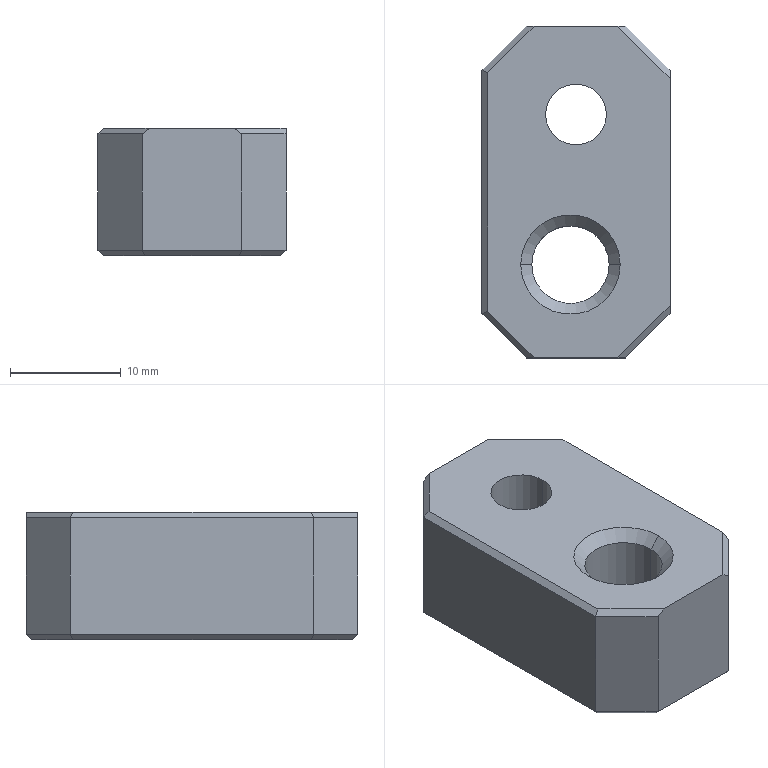Part | Creo | 1 solid | 34 faces | box 17 x 30 x 11.5 mm | volume 4458 mm3 | plane 24 | cylinder 6 | cone 4 | commonest cylinder face diameters 5.5 x2 7 x2 9.5 x2
STEP:
#1=CARTESIAN_POINT('',(-80.,-44.222,-93.5));
#2=VERTEX_POINT('',#1);
#3=CARTESIAN_POINT('',(-80.,-23.636,-93.5));
#4=VERTEX_POINT('',#3);
#5=CARTESIAN_POINT('',(-80.,-44.222,-93.5));
#6=DIRECTION('',(0.,1.,0.));
#7=VECTOR('',#6,20.586);
#8=LINE('',#5,#7);
#9=EDGE_CURVE('',#2,#4,#8,.T.);
#10=ORIENTED_EDGE('',*,*,#9,.F.);
#11=CARTESIAN_POINT('',(-84.707,-48.929,-93.5));
#12=VERTEX_POINT('',#11);
#13=CARTESIAN_POINT('',(-84.707,-48.929,-93.5));
#14=DIRECTION('',(0.7071,0.7071,0.));
#15=VECTOR('',#14,6.657);
#16=LINE('',#13,#15);
#17=EDGE_CURVE('',#12,#2,#16,.T.);
#18=ORIENTED_EDGE('',*,*,#17,.F.);
#19=CARTESIAN_POINT('',(-92.293,-48.929,-93.5));
#20=VERTEX_POINT('',#19);
#21=CARTESIAN_POINT('',(-92.293,-48.929,-93.5));
#22=DIRECTION('',(1.,0.,0.));
#23=VECTOR('',#22,7.586);
#24=LINE('',#21,#23);
#25=EDGE_CURVE('',#20,#12,#24,.T.);
#26=ORIENTED_EDGE('',*,*,#25,.F.);
#27=CARTESIAN_POINT('',(-96.5,-44.722,-93.5));
#28=VERTEX_POINT('',#27);
#29=CARTESIAN_POINT('',(-96.5,-44.722,-93.5));
#30=DIRECTION('',(0.7071,-0.7071,0.));
#31=VECTOR('',#30,5.95);
#32=LINE('',#29,#31);
#33=EDGE_CURVE('',#28,#20,#32,.T.);
#34=ORIENTED_EDGE('',*,*,#33,.F.);
#35=CARTESIAN_POINT('',(-96.5,-23.136,-93.5));
#36=VERTEX_POINT('',#35);
#37=CARTESIAN_POINT('',(-96.5,-44.722,-93.5));
#38=DIRECTION('',(0.,1.,0.));
#39=VECTOR('',#38,21.586);
#40=LINE('',#37,#39);
#41=EDGE_CURVE('',#28,#36,#40,.T.);
#42=ORIENTED_EDGE('',*,*,#41,.T.);
#43=CARTESIAN_POINT('',(-92.293,-18.929,-93.5));
#44=VERTEX_POINT('',#43);
#45=CARTESIAN_POINT('',(-92.293,-18.929,-93.5));
#46=DIRECTION('',(-0.7071,-0.7071,0.));
#47=VECTOR('',#46,5.95);
#48=LINE('',#45,#47);
#49=EDGE_CURVE('',#44,#36,#48,.T.);
#50=ORIENTED_EDGE('',*,*,#49,.F.);
#51=CARTESIAN_POINT('',(-84.707,-18.929,-93.5));
#52=VERTEX_POINT('',#51);
#53=CARTESIAN_POINT('',(-84.707,-18.929,-93.5));
#54=DIRECTION('',(-1.,0.,0.));
#55=VECTOR('',#54,7.586);
#56=LINE('',#53,#55);
#57=EDGE_CURVE('',#52,#44,#56,.T.);
#58=ORIENTED_EDGE('',*,*,#57,.F.);
#59=CARTESIAN_POINT('',(-80.,-23.636,-93.5));
#60=DIRECTION('',(-0.7071,0.7071,0.));
#61=VECTOR('',#60,6.657);
#62=LINE('',#59,#61);
#63=EDGE_CURVE('',#4,#52,#62,.T.);
#64=ORIENTED_EDGE('',*,*,#63,.F.);
#65=EDGE_LOOP('',(#10,#18,#26,#34,#42,#50,#58,#64));
#66=FACE_OUTER_BOUND('',#65,.F.);
#67=CARTESIAN_POINT('',(-91.25,-26.929,-93.5));
#68=VERTEX_POINT('',#67);
#69=CARTESIAN_POINT('',(-85.75,-26.929,-93.5));
#70=VERTEX_POINT('',#69);
#71=CARTESIAN_POINT('',(-88.5,-26.929,-93.5));
#72=DIRECTION('',(0.,0.,-1.));
#73=DIRECTION('',(-1.,0.,0.));
#74=AXIS2_PLACEMENT_3D('',#71,#72,#73);
#75=CIRCLE('',#74,2.75);
#76=EDGE_CURVE('',#68,#70,#75,.T.);
#77=ORIENTED_EDGE('',*,*,#76,.F.);
#78=CARTESIAN_POINT('',(-88.5,-26.929,-93.5));
#79=DIRECTION('',(0.,0.,-1.));
#80=DIRECTION('',(1.,0.,0.));
#81=AXIS2_PLACEMENT_3D('',#78,#79,#80);
#82=CIRCLE('',#81,2.75);
#83=EDGE_CURVE('',#70,#68,#82,.T.);
#84=ORIENTED_EDGE('',*,*,#83,.F.);
#85=EDGE_LOOP('',(#77,#84));
#86=FACE_BOUND('',#85,.F.);
#87=CARTESIAN_POINT('',(-84.5,-40.5,-93.5));
#88=VERTEX_POINT('',#87);
#89=CARTESIAN_POINT('',(-93.5,-40.5,-93.5));
#90=VERTEX_POINT('',#89);
#91=CARTESIAN_POINT('',(-89.,-40.5,-93.5));
#92=DIRECTION('',(0.,0.,-1.));
#93=DIRECTION('',(1.,0.,0.));
#94=AXIS2_PLACEMENT_3D('',#91,#92,#93);
#95=CIRCLE('',#94,4.5);
#96=EDGE_CURVE('',#88,#90,#95,.T.);
#97=ORIENTED_EDGE('',*,*,#96,.F.);
#98=CARTESIAN_POINT('',(-89.,-40.5,-93.5));
#99=DIRECTION('',(0.,0.,-1.));
#100=DIRECTION('',(-1.,0.,0.));
#101=AXIS2_PLACEMENT_3D('',#98,#99,#100);
#102=CIRCLE('',#101,4.5);
#103=EDGE_CURVE('',#90,#88,#102,.T.);
#104=ORIENTED_EDGE('',*,*,#103,.F.);
#105=EDGE_LOOP('',(#97,#104));
#106=FACE_BOUND('',#105,.F.);
#107=CARTESIAN_POINT('',(-88.428,-27.929,-93.5));
#108=DIRECTION('',(0.,0.,1.));
#109=DIRECTION('',(1.,0.,0.));
#110=AXIS2_PLACEMENT_3D('',#107,#108,#109);
#111=PLANE('',#110);
#112=ADVANCED_FACE('',(#66,#86,#106),#111,.T.);
#113=ORIENTED_EDGE('',*,*,#96,.T.);
#114=CARTESIAN_POINT('',(-92.5,-40.5,-94.5));
#115=VERTEX_POINT('',#114);
#116=CARTESIAN_POINT('',(-92.5,-40.5,-94.5));
#117=DIRECTION('',(-0.7071,0.,0.7071));
#118=VECTOR('',#117,1.414);
#119=LINE('',#116,#118);
#120=EDGE_CURVE('',#115,#90,#119,.T.);
#121=ORIENTED_EDGE('',*,*,#120,.F.);
#122=CARTESIAN_POINT('',(-85.5,-40.5,-94.5));
#123=VERTEX_POINT('',#122);
#124=CARTESIAN_POINT('',(-89.,-40.5,-94.5));
#125=DIRECTION('',(0.,0.,-1.));
#126=DIRECTION('',(1.,0.,0.));
#127=AXIS2_PLACEMENT_3D('',#124,#125,#126);
#128=CIRCLE('',#127,3.5);
#129=EDGE_CURVE('',#123,#115,#128,.T.);
#130=ORIENTED_EDGE('',*,*,#129,.F.);
#131=CARTESIAN_POINT('',(-85.5,-40.5,-94.5));
#132=DIRECTION('',(0.7071,0.,0.7071));
#133=VECTOR('',#132,1.414);
#134=LINE('',#131,#133);
#135=EDGE_CURVE('',#123,#88,#134,.T.);
#136=ORIENTED_EDGE('',*,*,#135,.T.);
#137=EDGE_LOOP('',(#113,#121,#130,#136));
#138=FACE_OUTER_BOUND('',#137,.F.);
#139=CARTESIAN_POINT('',(-89.,-40.5,-94.));
#140=DIRECTION('',(0.,0.,1.));
#141=DIRECTION('',(1.,0.,0.));
#142=AXIS2_PLACEMENT_3D('',#139,#140,#141);
#143=CONICAL_SURFACE('',#142,4.,45.);
#144=ADVANCED_FACE('',(#138),#143,.F.);
#145=ORIENTED_EDGE('',*,*,#103,.T.);
#146=ORIENTED_EDGE('',*,*,#135,.F.);
#147=CARTESIAN_POINT('',(-89.,-40.5,-94.5));
#148=DIRECTION('',(0.,0.,-1.));
#149=DIRECTION('',(-1.,0.,0.));
#150=AXIS2_PLACEMENT_3D('',#147,#148,#149);
#151=CIRCLE('',#150,3.5);
#152=EDGE_CURVE('',#115,#123,#151,.T.);
#153=ORIENTED_EDGE('',*,*,#152,.F.);
#154=ORIENTED_EDGE('',*,*,#120,.T.);
#155=EDGE_LOOP('',(#145,#146,#153,#154));
#156=FACE_OUTER_BOUND('',#155,.F.);
#157=CARTESIAN_POINT('',(-89.,-40.5,-94.));
#158=DIRECTION('',(0.,0.,1.));
#159=DIRECTION('',(1.,0.,0.));
#160=AXIS2_PLACEMENT_3D('',#157,#158,#159);
#161=CONICAL_SURFACE('',#160,4.,45.);
#162=ADVANCED_FACE('',(#156),#161,.F.);
#163=CARTESIAN_POINT('',(-85.5,-40.5,-104.));
#164=VERTEX_POINT('',#163);
#165=CARTESIAN_POINT('',(-92.5,-40.5,-104.));
#166=VERTEX_POINT('',#165);
#167=CARTESIAN_POINT('',(-89.,-40.5,-104.));
#168=DIRECTION('',(0.,0.,1.));
#169=DIRECTION('',(1.,0.,0.));
#170=AXIS2_PLACEMENT_3D('',#167,#168,#169);
#171=CIRCLE('',#170,3.5);
#172=EDGE_CURVE('',#164,#166,#171,.T.);
#173=ORIENTED_EDGE('',*,*,#172,.T.);
#174=CARTESIAN_POINT('',(-92.5,-40.5,-94.5));
#175=DIRECTION('',(0.,0.,-1.));
#176=VECTOR('',#175,9.5);
#177=LINE('',#174,#176);
#178=EDGE_CURVE('',#115,#166,#177,.T.);
#179=ORIENTED_EDGE('',*,*,#178,.F.);
#180=ORIENTED_EDGE('',*,*,#152,.T.);
#181=CARTESIAN_POINT('',(-85.5,-40.5,-94.5));
#182=DIRECTION('',(0.,0.,-1.));
#183=VECTOR('',#182,9.5);
#184=LINE('',#181,#183);
#185=EDGE_CURVE('',#123,#164,#184,.T.);
#186=ORIENTED_EDGE('',*,*,#185,.T.);
#187=EDGE_LOOP('',(#173,#179,#180,#186));
#188=FACE_OUTER_BOUND('',#187,.F.);
#189=CARTESIAN_POINT('',(-89.,-40.5,9.));
#190=DIRECTION('',(0.,0.,-1.));
#191=DIRECTION('',(1.,0.,0.));
#192=AXIS2_PLACEMENT_3D('',#189,#190,#191);
#193=CYLINDRICAL_SURFACE('',#192,3.5);
#194=ADVANCED_FACE('',(#188),#193,.F.);
#195=CARTESIAN_POINT('',(-84.5,-40.5,-105.));
#196=VERTEX_POINT('',#195);
#197=CARTESIAN_POINT('',(-93.5,-40.5,-105.));
#198=VERTEX_POINT('',#197);
#199=CARTESIAN_POINT('',(-89.,-40.5,-105.));
#200=DIRECTION('',(0.,0.,1.));
#201=DIRECTION('',(1.,0.,0.));
#202=AXIS2_PLACEMENT_3D('',#199,#200,#201);
#203=CIRCLE('',#202,4.5);
#204=EDGE_CURVE('',#196,#198,#203,.T.);
#205=ORIENTED_EDGE('',*,*,#204,.T.);
#206=CARTESIAN_POINT('',(-92.5,-40.5,-104.));
#207=DIRECTION('',(-0.7071,0.,-0.7071));
#208=VECTOR('',#207,1.414);
#209=LINE('',#206,#208);
#210=EDGE_CURVE('',#166,#198,#209,.T.);
#211=ORIENTED_EDGE('',*,*,#210,.F.);
#212=ORIENTED_EDGE('',*,*,#172,.F.);
#213=CARTESIAN_POINT('',(-85.5,-40.5,-104.));
#214=DIRECTION('',(0.7071,0.,-0.7071));
#215=VECTOR('',#214,1.414);
#216=LINE('',#213,#215);
#217=EDGE_CURVE('',#164,#196,#216,.T.);
#218=ORIENTED_EDGE('',*,*,#217,.T.);
#219=EDGE_LOOP('',(#205,#211,#212,#218));
#220=FACE_OUTER_BOUND('',#219,.F.);
#221=CARTESIAN_POINT('',(-89.,-40.5,-104.5));
#222=DIRECTION('',(0.,0.,-1.));
#223=DIRECTION('',(-1.,0.,0.));
#224=AXIS2_PLACEMENT_3D('',#221,#222,#223);
#225=CONICAL_SURFACE('',#224,4.,45.);
#226=ADVANCED_FACE('',(#220),#225,.F.);
#227=CARTESIAN_POINT('',(-80.5,-44.722,-105.));
#228=VERTEX_POINT('',#227);
#229=CARTESIAN_POINT('',(-80.5,-23.136,-105.));
#230=VERTEX_POINT('',#229);
#231=CARTESIAN_POINT('',(-80.5,-44.722,-105.));
#232=DIRECTION('',(0.,1.,0.));
#233=VECTOR('',#232,21.586);
#234=LINE('',#231,#233);
#235=EDGE_CURVE('',#228,#230,#234,.T.);
#236=ORIENTED_EDGE('',*,*,#235,.T.);
#237=CARTESIAN_POINT('',(-84.207,-19.429,-105.));
#238=VERTEX_POINT('',#237);
#239=CARTESIAN_POINT('',(-84.207,-19.429,-105.));
#240=DIRECTION('',(0.7071,-0.7071,0.));
#241=VECTOR('',#240,5.243);
#242=LINE('',#239,#241);
#243=EDGE_CURVE('',#238,#230,#242,.T.);
#244=ORIENTED_EDGE('',*,*,#243,.F.);
#245=CARTESIAN_POINT('',(-92.793,-19.429,-105.));
#246=VERTEX_POINT('',#245);
#247=CARTESIAN_POINT('',(-84.207,-19.429,-105.));
#248=DIRECTION('',(-1.,0.,0.));
#249=VECTOR('',#248,8.586);
#250=LINE('',#247,#249);
#251=EDGE_CURVE('',#238,#246,#250,.T.);
#252=ORIENTED_EDGE('',*,*,#251,.T.);
#253=CARTESIAN_POINT('',(-96.5,-23.136,-105.));
#254=VERTEX_POINT('',#253);
#255=CARTESIAN_POINT('',(-96.5,-23.136,-105.));
#256=DIRECTION('',(0.7071,0.7071,0.));
#257=VECTOR('',#256,5.243);
#258=LINE('',#255,#257);
#259=EDGE_CURVE('',#254,#246,#258,.T.);
#260=ORIENTED_EDGE('',*,*,#259,.F.);
#261=CARTESIAN_POINT('',(-96.5,-44.722,-105.));
#262=VERTEX_POINT('',#261);
#263=CARTESIAN_POINT('',(-96.5,-23.136,-105.));
#264=DIRECTION('',(0.,-1.,0.));
#265=VECTOR('',#264,21.586);
#266=LINE('',#263,#265);
#267=EDGE_CURVE('',#254,#262,#266,.T.);
#268=ORIENTED_EDGE('',*,*,#267,.T.);
#269=CARTESIAN_POINT('',(-92.793,-48.429,-105.));
#270=VERTEX_POINT('',#269);
#271=CARTESIAN_POINT('',(-92.793,-48.429,-105.));
#272=DIRECTION('',(-0.7071,0.7071,0.));
#273=VECTOR('',#272,5.243);
#274=LINE('',#271,#273);
#275=EDGE_CURVE('',#270,#262,#274,.T.);
#276=ORIENTED_EDGE('',*,*,#275,.F.);
#277=CARTESIAN_POINT('',(-84.207,-48.429,-105.));
#278=VERTEX_POINT('',#277);
#279=CARTESIAN_POINT('',(-92.793,-48.429,-105.));
#280=DIRECTION('',(1.,0.,0.));
#281=VECTOR('',#280,8.586);
#282=LINE('',#279,#281);
#283=EDGE_CURVE('',#270,#278,#282,.T.);
#284=ORIENTED_EDGE('',*,*,#283,.T.);
#285=CARTESIAN_POINT('',(-80.5,-44.722,-105.));
#286=DIRECTION('',(-0.7071,-0.7071,0.));
#287=VECTOR('',#286,5.243);
#288=LINE('',#285,#287);
#289=EDGE_CURVE('',#228,#278,#288,.T.);
#290=ORIENTED_EDGE('',*,*,#289,.F.);
#291=EDGE_LOOP('',(#236,#244,#252,#260,#268,#276,#284,#290));
#292=FACE_OUTER_BOUND('',#291,.F.);
#293=CARTESIAN_POINT('',(-83.75,-26.929,-105.));
#294=VERTEX_POINT('',#293);
#295=CARTESIAN_POINT('',(-93.25,-26.929,-105.));
#296=VERTEX_POINT('',#295);
#297=CARTESIAN_POINT('',(-88.5,-26.929,-105.));
#298=DIRECTION('',(0.,0.,1.));
#299=DIRECTION('',(1.,0.,0.));
#300=AXIS2_PLACEMENT_3D('',#297,#298,#299);
#301=CIRCLE('',#300,4.75);
#302=EDGE_CURVE('',#294,#296,#301,.T.);
#303=ORIENTED_EDGE('',*,*,#302,.F.);
#304=CARTESIAN_POINT('',(-88.5,-26.929,-105.));
#305=DIRECTION('',(0.,0.,1.));
#306=DIRECTION('',(-1.,0.,0.));
#307=AXIS2_PLACEMENT_3D('',#304,#305,#306);
#308=CIRCLE('',#307,4.75);
#309=EDGE_CURVE('',#296,#294,#308,.T.);
#310=ORIENTED_EDGE('',*,*,#309,.F.);
#311=EDGE_LOOP('',(#303,#310));
#312=FACE_BOUND('',#311,.F.);
#313=CARTESIAN_POINT('',(-89.,-40.5,-105.));
#314=DIRECTION('',(0.,0.,1.));
#315=DIRECTION('',(-1.,0.,0.));
#316=AXIS2_PLACEMENT_3D('',#313,#314,#315);
#317=CIRCLE('',#316,4.5);
#318=EDGE_CURVE('',#198,#196,#317,.T.);
#319=ORIENTED_EDGE('',*,*,#318,.F.);
#320=ORIENTED_EDGE('',*,*,#204,.F.);
#321=EDGE_LOOP('',(#319,#320));
#322=FACE_BOUND('',#321,.F.);
#323=CARTESIAN_POINT('',(-176.,-14.505,-105.));
#324=DIRECTION('',(0.,0.,-1.));
#325=DIRECTION('',(-1.,0.,0.));
#326=AXIS2_PLACEMENT_3D('',#323,#324,#325);
#327=PLANE('',#326);
#328=ADVANCED_FACE('',(#292,#312,#322),#327,.T.);
#329=ORIENTED_EDGE('',*,*,#318,.T.);
#330=ORIENTED_EDGE('',*,*,#217,.F.);
#331=CARTESIAN_POINT('',(-89.,-40.5,-104.));
#332=DIRECTION('',(0.,0.,1.));
#333=DIRECTION('',(-1.,0.,0.));
#334=AXIS2_PLACEMENT_3D('',#331,#332,#333);
#335=CIRCLE('',#334,3.5);
#336=EDGE_CURVE('',#166,#164,#335,.T.);
#337=ORIENTED_EDGE('',*,*,#336,.F.);
#338=ORIENTED_EDGE('',*,*,#210,.T.);
#339=EDGE_LOOP('',(#329,#330,#337,#338));
#340=FACE_OUTER_BOUND('',#339,.F.);
#341=CARTESIAN_POINT('',(-89.,-40.5,-104.5));
#342=DIRECTION('',(0.,0.,-1.));
#343=DIRECTION('',(-1.,0.,0.));
#344=AXIS2_PLACEMENT_3D('',#341,#342,#343);
#345=CONICAL_SURFACE('',#344,4.,45.);
#346=ADVANCED_FACE('',(#340),#345,.F.);
#347=ORIENTED_EDGE('',*,*,#336,.T.);
#348=ORIENTED_EDGE('',*,*,#185,.F.);
#349=ORIENTED_EDGE('',*,*,#129,.T.);
#350=ORIENTED_EDGE('',*,*,#178,.T.);
#351=EDGE_LOOP('',(#347,#348,#349,#350));
#352=FACE_OUTER_BOUND('',#351,.F.);
#353=CARTESIAN_POINT('',(-89.,-40.5,9.));
#354=DIRECTION('',(0.,0.,-1.));
#355=DIRECTION('',(1.,0.,0.));
#356=AXIS2_PLACEMENT_3D('',#353,#354,#355);
#357=CYLINDRICAL_SURFACE('',#356,3.5);
#358=ADVANCED_FACE('',(#352),#357,.F.);
#359=CARTESIAN_POINT('',(-93.25,-26.929,-99.));
#360=VERTEX_POINT('',#359);
#361=CARTESIAN_POINT('',(-83.75,-26.929,-99.));
#362=VERTEX_POINT('',#361);
#363=CARTESIAN_POINT('',(-88.5,-26.929,-99.));
#364=DIRECTION('',(0.,0.,-1.));
#365=DIRECTION('',(-1.,0.,0.));
#366=AXIS2_PLACEMENT_3D('',#363,#364,#365);
#367=CIRCLE('',#366,4.75);
#368=EDGE_CURVE('',#360,#362,#367,.T.);
#369=ORIENTED_EDGE('',*,*,#368,.T.);
#370=CARTESIAN_POINT('',(-83.75,-26.929,-99.));
#371=DIRECTION('',(0.,0.,-1.));
#372=VECTOR('',#371,6.);
#373=LINE('',#370,#372);
#374=EDGE_CURVE('',#362,#294,#373,.T.);
#375=ORIENTED_EDGE('',*,*,#374,.T.);
#376=ORIENTED_EDGE('',*,*,#302,.T.);
#377=CARTESIAN_POINT('',(-93.25,-26.929,-99.));
#378=DIRECTION('',(0.,0.,-1.));
#379=VECTOR('',#378,6.);
#380=LINE('',#377,#379);
#381=EDGE_CURVE('',#360,#296,#380,.T.);
#382=ORIENTED_EDGE('',*,*,#381,.F.);
#383=EDGE_LOOP('',(#369,#375,#376,#382));
#384=FACE_OUTER_BOUND('',#383,.F.);
#385=CARTESIAN_POINT('',(-88.5,-26.929,-105.));
#386=DIRECTION('',(0.,0.,-1.));
#387=DIRECTION('',(-1.,0.,0.));
#388=AXIS2_PLACEMENT_3D('',#385,#386,#387);
#389=CYLINDRICAL_SURFACE('',#388,4.75);
#390=ADVANCED_FACE('',(#384),#389,.F.);
#391=CARTESIAN_POINT('',(-88.5,-26.929,-99.));
#392=DIRECTION('',(0.,0.,-1.));
#393=DIRECTION('',(1.,0.,0.));
#394=AXIS2_PLACEMENT_3D('',#391,#392,#393);
#395=CIRCLE('',#394,4.75);
#396=EDGE_CURVE('',#362,#360,#395,.T.);
#397=ORIENTED_EDGE('',*,*,#396,.F.);
#398=ORIENTED_EDGE('',*,*,#368,.F.);
#399=EDGE_LOOP('',(#397,#398));
#400=FACE_OUTER_BOUND('',#399,.F.);
#401=CARTESIAN_POINT('',(-85.75,-26.929,-99.));
#402=VERTEX_POINT('',#401);
#403=CARTESIAN_POINT('',(-91.25,-26.929,-99.));
#404=VERTEX_POINT('',#403);
#405=CARTESIAN_POINT('',(-88.5,-26.929,-99.));
#406=DIRECTION('',(0.,0.,1.));
#407=DIRECTION('',(1.,0.,0.));
#408=AXIS2_PLACEMENT_3D('',#405,#406,#407);
#409=CIRCLE('',#408,2.75);
#410=EDGE_CURVE('',#402,#404,#409,.T.);
#411=ORIENTED_EDGE('',*,*,#410,.F.);
#412=CARTESIAN_POINT('',(-88.5,-26.929,-99.));
#413=DIRECTION('',(0.,0.,1.));
#414=DIRECTION('',(-1.,0.,0.));
#415=AXIS2_PLACEMENT_3D('',#412,#413,#414);
#416=CIRCLE('',#415,2.75);
#417=EDGE_CURVE('',#404,#402,#416,.T.);
#418=ORIENTED_EDGE('',*,*,#417,.F.);
#419=EDGE_LOOP('',(#411,#418));
#420=FACE_BOUND('',#419,.F.);
#421=CARTESIAN_POINT('',(-88.5,-31.679,-99.));
#422=DIRECTION('',(0.,0.,1.));
#423=DIRECTION('',(1.,0.,0.));
#424=AXIS2_PLACEMENT_3D('',#421,#422,#423);
#425=PLANE('',#424);
#426=ADVANCED_FACE('',(#400,#420),#425,.F.);
#427=ORIENTED_EDGE('',*,*,#76,.T.);
#428=CARTESIAN_POINT('',(-85.75,-26.929,-93.5));
#429=DIRECTION('',(0.,0.,-1.));
#430=VECTOR('',#429,5.5);
#431=LINE('',#428,#430);
#432=EDGE_CURVE('',#70,#402,#431,.T.);
#433=ORIENTED_EDGE('',*,*,#432,.T.);
#434=ORIENTED_EDGE('',*,*,#410,.T.);
#435=CARTESIAN_POINT('',(-91.25,-26.929,-93.5));
#436=DIRECTION('',(0.,0.,-1.));
#437=VECTOR('',#436,5.5);
#438=LINE('',#435,#437);
#439=EDGE_CURVE('',#68,#404,#438,.T.);
#440=ORIENTED_EDGE('',*,*,#439,.F.);
#441=EDGE_LOOP('',(#427,#433,#434,#440));
#442=FACE_OUTER_BOUND('',#441,.F.);
#443=CARTESIAN_POINT('',(-88.5,-26.929,-105.));
#444=DIRECTION('',(0.,0.,-1.));
#445=DIRECTION('',(-1.,0.,0.));
#446=AXIS2_PLACEMENT_3D('',#443,#444,#445);
#447=CYLINDRICAL_SURFACE('',#446,2.75);
#448=ADVANCED_FACE('',(#442),#447,.F.);
#449=ORIENTED_EDGE('',*,*,#83,.T.);
#450=ORIENTED_EDGE('',*,*,#439,.T.);
#451=ORIENTED_EDGE('',*,*,#417,.T.);
#452=ORIENTED_EDGE('',*,*,#432,.F.);
#453=EDGE_LOOP('',(#449,#450,#451,#452));
#454=FACE_OUTER_BOUND('',#453,.F.);
#455=CARTESIAN_POINT('',(-88.5,-26.929,-105.));
#456=DIRECTION('',(0.,0.,-1.));
#457=DIRECTION('',(-1.,0.,0.));
#458=AXIS2_PLACEMENT_3D('',#455,#456,#457);
#459=CYLINDRICAL_SURFACE('',#458,2.75);
#460=ADVANCED_FACE('',(#454),#459,.F.);
#461=ORIENTED_EDGE('',*,*,#396,.T.);
#462=ORIENTED_EDGE('',*,*,#381,.T.);
#463=ORIENTED_EDGE('',*,*,#309,.T.);
#464=ORIENTED_EDGE('',*,*,#374,.F.);
#465=EDGE_LOOP('',(#461,#462,#463,#464));
#466=FACE_OUTER_BOUND('',#465,.F.);
#467=CARTESIAN_POINT('',(-88.5,-26.929,-105.));
#468=DIRECTION('',(0.,0.,-1.));
#469=DIRECTION('',(-1.,0.,0.));
#470=AXIS2_PLACEMENT_3D('',#467,#468,#469);
#471=CYLINDRICAL_SURFACE('',#470,4.75);
#472=ADVANCED_FACE('',(#466),#471,.F.);
#473=CARTESIAN_POINT('',(-80.,-22.929,-104.5));
#474=VERTEX_POINT('',#473);
#475=CARTESIAN_POINT('',(-80.,-22.929,-104.5));
#476=DIRECTION('',(-0.6786,-0.2811,-0.6786));
#477=VECTOR('',#476,0.7368);
#478=LINE('',#475,#477);
#479=EDGE_CURVE('',#474,#230,#478,.T.);
#480=ORIENTED_EDGE('',*,*,#479,.T.);
#481=ORIENTED_EDGE('',*,*,#235,.F.);
#482=CARTESIAN_POINT('',(-80.,-44.929,-104.5));
#483=VERTEX_POINT('',#482);
#484=CARTESIAN_POINT('',(-80.5,-44.722,-105.));
#485=DIRECTION('',(0.6786,-0.2811,0.6786));
#486=VECTOR('',#485,0.7368);
#487=LINE('',#484,#486);
#488=EDGE_CURVE('',#228,#483,#487,.T.);
#489=ORIENTED_EDGE('',*,*,#488,.T.);
#490=CARTESIAN_POINT('',(-80.,-22.929,-104.5));
#491=DIRECTION('',(0.,-1.,0.));
#492=VECTOR('',#491,22.);
#493=LINE('',#490,#492);
#494=EDGE_CURVE('',#474,#483,#493,.T.);
#495=ORIENTED_EDGE('',*,*,#494,.F.);
#496=EDGE_LOOP('',(#480,#481,#489,#495));
#497=FACE_OUTER_BOUND('',#496,.F.);
#498=CARTESIAN_POINT('',(-80.,-27.929,-104.5));
#499=DIRECTION('',(-0.7071,0.,0.7071));
#500=DIRECTION('',(0.,1.,0.));
#501=AXIS2_PLACEMENT_3D('',#498,#499,#500);
#502=PLANE('',#501);
#503=ADVANCED_FACE('',(#497),#502,.F.);
#504=CARTESIAN_POINT('',(-84.,-18.929,-104.5));
#505=VERTEX_POINT('',#504);
#506=CARTESIAN_POINT('',(-84.,-18.929,-104.5));
#507=DIRECTION('',(0.7071,-0.7071,0.));
#508=VECTOR('',#507,5.657);
#509=LINE('',#506,#508);
#510=EDGE_CURVE('',#505,#474,#509,.T.);
#511=ORIENTED_EDGE('',*,*,#510,.F.);
#512=CARTESIAN_POINT('',(-84.207,-19.429,-105.));
#513=DIRECTION('',(0.2811,0.6786,0.6786));
#514=VECTOR('',#513,0.7368);
#515=LINE('',#512,#514);
#516=EDGE_CURVE('',#238,#505,#515,.T.);
#517=ORIENTED_EDGE('',*,*,#516,.F.);
#518=ORIENTED_EDGE('',*,*,#243,.T.);
#519=ORIENTED_EDGE('',*,*,#479,.F.);
#520=EDGE_LOOP('',(#511,#517,#518,#519));
#521=FACE_OUTER_BOUND('',#520,.F.);
#522=CARTESIAN_POINT('',(-132.566,28.929,-105.));
#523=DIRECTION('',(0.5,0.5,-0.7071));
#524=DIRECTION('',(-0.7071,0.7071,0.));
#525=AXIS2_PLACEMENT_3D('',#522,#523,#524);
#526=PLANE('',#525);
#527=ADVANCED_FACE('',(#521),#526,.T.);
#528=CARTESIAN_POINT('',(-80.,-22.929,-94.));
#529=VERTEX_POINT('',#528);
#530=CARTESIAN_POINT('',(-80.,-22.929,-94.));
#531=DIRECTION('',(0.,0.,-1.));
#532=VECTOR('',#531,10.5);
#533=LINE('',#530,#532);
#534=EDGE_CURVE('',#529,#474,#533,.T.);
#535=ORIENTED_EDGE('',*,*,#534,.F.);
#536=CARTESIAN_POINT('',(-84.,-18.929,-94.));
#537=VERTEX_POINT('',#536);
#538=CARTESIAN_POINT('',(-80.,-22.929,-94.));
#539=DIRECTION('',(-0.7071,0.7071,0.));
#540=VECTOR('',#539,5.657);
#541=LINE('',#538,#540);
#542=EDGE_CURVE('',#529,#537,#541,.T.);
#543=ORIENTED_EDGE('',*,*,#542,.T.);
#544=CARTESIAN_POINT('',(-84.,-18.929,-104.5));
#545=DIRECTION('',(0.,0.,1.));
#546=VECTOR('',#545,10.5);
#547=LINE('',#544,#546);
#548=EDGE_CURVE('',#505,#537,#547,.T.);
#549=ORIENTED_EDGE('',*,*,#548,.F.);
#550=ORIENTED_EDGE('',*,*,#510,.T.);
#551=EDGE_LOOP('',(#535,#543,#549,#550));
#552=FACE_OUTER_BOUND('',#551,.F.);
#553=CARTESIAN_POINT('',(-84.,-18.929,-93.5));
#554=DIRECTION('',(-0.7071,-0.7071,0.));
#555=DIRECTION('',(0.,0.,-1.));
#556=AXIS2_PLACEMENT_3D('',#553,#554,#555);
#557=PLANE('',#556);
#558=ADVANCED_FACE('',(#552),#557,.F.);
#559=CARTESIAN_POINT('',(-80.,-44.929,-94.));
#560=VERTEX_POINT('',#559);
#561=CARTESIAN_POINT('',(-80.,-44.929,-104.5));
#562=DIRECTION('',(0.,0.,1.));
#563=VECTOR('',#562,10.5);
#564=LINE('',#561,#563);
#565=EDGE_CURVE('',#483,#560,#564,.T.);
#566=ORIENTED_EDGE('',*,*,#565,.T.);
#567=CARTESIAN_POINT('',(-80.,-44.929,-94.));
#568=DIRECTION('',(0.,0.8165,0.5774));
#569=VECTOR('',#568,0.866);
#570=LINE('',#567,#569);
#571=EDGE_CURVE('',#560,#2,#570,.T.);
#572=ORIENTED_EDGE('',*,*,#571,.T.);
#573=ORIENTED_EDGE('',*,*,#9,.T.);
#574=CARTESIAN_POINT('',(-80.,-23.636,-93.5));
#575=DIRECTION('',(0.,0.8165,-0.5774));
#576=VECTOR('',#575,0.866);
#577=LINE('',#574,#576);
#578=EDGE_CURVE('',#4,#529,#577,.T.);
#579=ORIENTED_EDGE('',*,*,#578,.T.);
#580=ORIENTED_EDGE('',*,*,#534,.T.);
#581=ORIENTED_EDGE('',*,*,#494,.T.);
#582=EDGE_LOOP('',(#566,#572,#573,#579,#580,#581));
#583=FACE_OUTER_BOUND('',#582,.F.);
#584=CARTESIAN_POINT('',(-80.,-27.929,-93.5));
#585=DIRECTION('',(1.,0.,0.));
#586=DIRECTION('',(0.,0.,-1.));
#587=AXIS2_PLACEMENT_3D('',#584,#585,#586);
#588=PLANE('',#587);
#589=ADVANCED_FACE('',(#583),#588,.T.);
#590=ORIENTED_EDGE('',*,*,#565,.F.);
#591=CARTESIAN_POINT('',(-84.,-48.929,-104.5));
#592=VERTEX_POINT('',#591);
#593=CARTESIAN_POINT('',(-80.,-44.929,-104.5));
#594=DIRECTION('',(-0.7071,-0.7071,0.));
#595=VECTOR('',#594,5.657);
#596=LINE('',#593,#595);
#597=EDGE_CURVE('',#483,#592,#596,.T.);
#598=ORIENTED_EDGE('',*,*,#597,.T.);
#599=CARTESIAN_POINT('',(-84.,-48.929,-94.));
#600=VERTEX_POINT('',#599);
#601=CARTESIAN_POINT('',(-84.,-48.929,-94.));
#602=DIRECTION('',(0.,0.,-1.));
#603=VECTOR('',#602,10.5);
#604=LINE('',#601,#603);
#605=EDGE_CURVE('',#600,#592,#604,.T.);
#606=ORIENTED_EDGE('',*,*,#605,.F.);
#607=CARTESIAN_POINT('',(-84.,-48.929,-94.));
#608=DIRECTION('',(0.7071,0.7071,0.));
#609=VECTOR('',#608,5.657);
#610=LINE('',#607,#609);
#611=EDGE_CURVE('',#600,#560,#610,.T.);
#612=ORIENTED_EDGE('',*,*,#611,.T.);
#613=EDGE_LOOP('',(#590,#598,#606,#612));
#614=FACE_OUTER_BOUND('',#613,.F.);
#615=CARTESIAN_POINT('',(-80.,-44.929,-93.5));
#616=DIRECTION('',(-0.7071,0.7071,0.));
#617=DIRECTION('',(0.,0.,-1.));
#618=AXIS2_PLACEMENT_3D('',#615,#616,#617);
#619=PLANE('',#618);
#620=ADVANCED_FACE('',(#614),#619,.F.);
#621=ORIENTED_EDGE('',*,*,#289,.T.);
#622=CARTESIAN_POINT('',(-84.,-48.929,-104.5));
#623=DIRECTION('',(-0.2811,0.6786,-0.6786));
#624=VECTOR('',#623,0.7368);
#625=LINE('',#622,#624);
#626=EDGE_CURVE('',#592,#278,#625,.T.);
#627=ORIENTED_EDGE('',*,*,#626,.F.);
#628=ORIENTED_EDGE('',*,*,#597,.F.);
#629=ORIENTED_EDGE('',*,*,#488,.F.);
#630=EDGE_LOOP('',(#621,#627,#628,#629));
#631=FACE_OUTER_BOUND('',#630,.F.);
#632=CARTESIAN_POINT('',(-113.141,-77.363,-105.));
#633=DIRECTION('',(0.5,-0.5,-0.7071));
#634=DIRECTION('',(0.7071,0.7071,0.));
#635=AXIS2_PLACEMENT_3D('',#632,#633,#634);
#636=PLANE('',#635);
#637=ADVANCED_FACE('',(#631),#636,.T.);
#638=CARTESIAN_POINT('',(-93.,-48.929,-104.5));
#639=VERTEX_POINT('',#638);
#640=CARTESIAN_POINT('',(-84.,-48.929,-104.5));
#641=DIRECTION('',(-1.,0.,0.));
#642=VECTOR('',#641,9.);
#643=LINE('',#640,#642);
#644=EDGE_CURVE('',#592,#639,#643,.T.);
#645=ORIENTED_EDGE('',*,*,#644,.F.);
#646=ORIENTED_EDGE('',*,*,#626,.T.);
#647=ORIENTED_EDGE('',*,*,#283,.F.);
#648=CARTESIAN_POINT('',(-92.793,-48.429,-105.));
#649=DIRECTION('',(-0.2811,-0.6786,0.6786));
#650=VECTOR('',#649,0.7368);
#651=LINE('',#648,#650);
#652=EDGE_CURVE('',#270,#639,#651,.T.);
#653=ORIENTED_EDGE('',*,*,#652,.T.);
#654=EDGE_LOOP('',(#645,#646,#647,#653));
#655=FACE_OUTER_BOUND('',#654,.F.);
#656=CARTESIAN_POINT('',(33.,-48.929,-104.5));
#657=DIRECTION('',(0.,0.7071,0.7071));
#658=DIRECTION('',(1.,0.,0.));
#659=AXIS2_PLACEMENT_3D('',#656,#657,#658);
#660=PLANE('',#659);
#661=ADVANCED_FACE('',(#655),#660,.F.);
#662=ORIENTED_EDGE('',*,*,#25,.T.);
#663=CARTESIAN_POINT('',(-84.707,-48.929,-93.5));
#664=DIRECTION('',(0.8165,0.,-0.5774));
#665=VECTOR('',#664,0.866);
#666=LINE('',#663,#665);
#667=EDGE_CURVE('',#12,#600,#666,.T.);
#668=ORIENTED_EDGE('',*,*,#667,.T.);
#669=ORIENTED_EDGE('',*,*,#605,.T.);
#670=ORIENTED_EDGE('',*,*,#644,.T.);
#671=CARTESIAN_POINT('',(-93.,-48.929,-94.));
#672=VERTEX_POINT('',#671);
#673=CARTESIAN_POINT('',(-93.,-48.929,-104.5));
#674=DIRECTION('',(0.,0.,1.));
#675=VECTOR('',#674,10.5);
#676=LINE('',#673,#675);
#677=EDGE_CURVE('',#639,#672,#676,.T.);
#678=ORIENTED_EDGE('',*,*,#677,.T.);
#679=CARTESIAN_POINT('',(-93.,-48.929,-94.));
#680=DIRECTION('',(0.8165,0.,0.5774));
#681=VECTOR('',#680,0.866);
#682=LINE('',#679,#681);
#683=EDGE_CURVE('',#672,#20,#682,.T.);
#684=ORIENTED_EDGE('',*,*,#683,.T.);
#685=EDGE_LOOP('',(#662,#668,#669,#670,#678,#684));
#686=FACE_OUTER_BOUND('',#685,.F.);
#687=CARTESIAN_POINT('',(33.,-48.929,-105.096));
#688=DIRECTION('',(0.,-1.,0.));
#689=DIRECTION('',(0.,0.,1.));
#690=AXIS2_PLACEMENT_3D('',#687,#688,#689);
#691=PLANE('',#690);
#692=ADVANCED_FACE('',(#686),#691,.T.);
#693=ORIENTED_EDGE('',*,*,#667,.F.);
#694=ORIENTED_EDGE('',*,*,#17,.T.);
#695=ORIENTED_EDGE('',*,*,#571,.F.);
#696=ORIENTED_EDGE('',*,*,#611,.F.);
#697=EDGE_LOOP('',(#693,#694,#695,#696));
#698=FACE_OUTER_BOUND('',#697,.F.);
#699=CARTESIAN_POINT('',(-76.068,-40.29,-93.5));
#700=DIRECTION('',(0.5,-0.5,0.7071));
#701=DIRECTION('',(-0.7071,-0.7071,0.));
#702=AXIS2_PLACEMENT_3D('',#699,#700,#701);
#703=PLANE('',#702);
#704=ADVANCED_FACE('',(#698),#703,.T.);
#705=ORIENTED_EDGE('',*,*,#677,.F.);
#706=CARTESIAN_POINT('',(-97.,-44.929,-104.5));
#707=VERTEX_POINT('',#706);
#708=CARTESIAN_POINT('',(-93.,-48.929,-104.5));
#709=DIRECTION('',(-0.7071,0.7071,0.));
#710=VECTOR('',#709,5.657);
#711=LINE('',#708,#710);
#712=EDGE_CURVE('',#639,#707,#711,.T.);
#713=ORIENTED_EDGE('',*,*,#712,.T.);
#714=CARTESIAN_POINT('',(-97.,-44.929,-94.));
#715=VERTEX_POINT('',#714);
#716=CARTESIAN_POINT('',(-97.,-44.929,-94.));
#717=DIRECTION('',(0.,0.,-1.));
#718=VECTOR('',#717,10.5);
#719=LINE('',#716,#718);
#720=EDGE_CURVE('',#715,#707,#719,.T.);
#721=ORIENTED_EDGE('',*,*,#720,.F.);
#722=CARTESIAN_POINT('',(-97.,-44.929,-94.));
#723=DIRECTION('',(0.7071,-0.7071,0.));
#724=VECTOR('',#723,5.657);
#725=LINE('',#722,#724);
#726=EDGE_CURVE('',#715,#672,#725,.T.);
#727=ORIENTED_EDGE('',*,*,#726,.T.);
#728=EDGE_LOOP('',(#705,#713,#721,#727));
#729=FACE_OUTER_BOUND('',#728,.F.);
#730=CARTESIAN_POINT('',(-93.,-48.929,-105.096));
#731=DIRECTION('',(0.7071,0.7071,0.));
#732=DIRECTION('',(0.,0.,-1.));
#733=AXIS2_PLACEMENT_3D('',#730,#731,#732);
#734=PLANE('',#733);
#735=ADVANCED_FACE('',(#729),#734,.F.);
#736=ORIENTED_EDGE('',*,*,#652,.F.);
#737=ORIENTED_EDGE('',*,*,#275,.T.);
#738=CARTESIAN_POINT('',(-97.,-44.929,-104.5));
#739=DIRECTION('',(0.6786,0.2811,-0.6786));
#740=VECTOR('',#739,0.7368);
#741=LINE('',#738,#740);
#742=EDGE_CURVE('',#707,#262,#741,.T.);
#743=ORIENTED_EDGE('',*,*,#742,.F.);
#744=ORIENTED_EDGE('',*,*,#712,.F.);
#745=EDGE_LOOP('',(#736,#737,#743,#744));
#746=FACE_OUTER_BOUND('',#745,.F.);
#747=CARTESIAN_POINT('',(-151.359,10.137,-105.));
#748=DIRECTION('',(-0.5,-0.5,-0.7071));
#749=DIRECTION('',(0.7071,-0.7071,0.));
#750=AXIS2_PLACEMENT_3D('',#747,#748,#749);
#751=PLANE('',#750);
#752=ADVANCED_FACE('',(#746),#751,.T.);
#753=CARTESIAN_POINT('',(-97.,-22.929,-104.5));
#754=VERTEX_POINT('',#753);
#755=CARTESIAN_POINT('',(-97.,-44.929,-104.5));
#756=DIRECTION('',(0.,1.,0.));
#757=VECTOR('',#756,22.);
#758=LINE('',#755,#757);
#759=EDGE_CURVE('',#707,#754,#758,.T.);
#760=ORIENTED_EDGE('',*,*,#759,.F.);
#761=ORIENTED_EDGE('',*,*,#742,.T.);
#762=ORIENTED_EDGE('',*,*,#267,.F.);
#763=CARTESIAN_POINT('',(-96.5,-23.136,-105.));
#764=DIRECTION('',(-0.6786,0.2811,0.6786));
#765=VECTOR('',#764,0.7368);
#766=LINE('',#763,#765);
#767=EDGE_CURVE('',#254,#754,#766,.T.);
#768=ORIENTED_EDGE('',*,*,#767,.T.);
#769=EDGE_LOOP('',(#760,#761,#762,#768));
#770=FACE_OUTER_BOUND('',#769,.F.);
#771=CARTESIAN_POINT('',(-97.,-40.429,-104.5));
#772=DIRECTION('',(0.7071,0.,0.7071));
#773=DIRECTION('',(0.,-1.,0.));
#774=AXIS2_PLACEMENT_3D('',#771,#772,#773);
#775=PLANE('',#774);
#776=ADVANCED_FACE('',(#770),#775,.F.);
#777=ORIENTED_EDGE('',*,*,#720,.T.);
#778=ORIENTED_EDGE('',*,*,#759,.T.);
#779=CARTESIAN_POINT('',(-97.,-22.929,-94.));
#780=VERTEX_POINT('',#779);
#781=CARTESIAN_POINT('',(-97.,-22.929,-104.5));
#782=DIRECTION('',(0.,0.,1.));
#783=VECTOR('',#782,10.5);
#784=LINE('',#781,#783);
#785=EDGE_CURVE('',#754,#780,#784,.T.);
#786=ORIENTED_EDGE('',*,*,#785,.T.);
#787=CARTESIAN_POINT('',(-97.,-22.929,-94.));
#788=DIRECTION('',(0.,-1.,0.));
#789=VECTOR('',#788,22.);
#790=LINE('',#787,#789);
#791=EDGE_CURVE('',#780,#715,#790,.T.);
#792=ORIENTED_EDGE('',*,*,#791,.T.);
#793=EDGE_LOOP('',(#777,#778,#786,#792));
#794=FACE_OUTER_BOUND('',#793,.F.);
#795=CARTESIAN_POINT('',(-97.,-40.429,-105.096));
#796=DIRECTION('',(-1.,0.,0.));
#797=DIRECTION('',(0.,0.,1.));
#798=AXIS2_PLACEMENT_3D('',#795,#796,#797);
#799=PLANE('',#798);
#800=ADVANCED_FACE('',(#794),#799,.T.);
#801=ORIENTED_EDGE('',*,*,#785,.F.);
#802=CARTESIAN_POINT('',(-93.,-18.929,-104.5));
#803=VERTEX_POINT('',#802);
#804=CARTESIAN_POINT('',(-97.,-22.929,-104.5));
#805=DIRECTION('',(0.7071,0.7071,0.));
#806=VECTOR('',#805,5.657);
#807=LINE('',#804,#806);
#808=EDGE_CURVE('',#754,#803,#807,.T.);
#809=ORIENTED_EDGE('',*,*,#808,.T.);
#810=CARTESIAN_POINT('',(-93.,-18.929,-94.));
#811=VERTEX_POINT('',#810);
#812=CARTESIAN_POINT('',(-93.,-18.929,-94.));
#813=DIRECTION('',(0.,0.,-1.));
#814=VECTOR('',#813,10.5);
#815=LINE('',#812,#814);
#816=EDGE_CURVE('',#811,#803,#815,.T.);
#817=ORIENTED_EDGE('',*,*,#816,.F.);
#818=CARTESIAN_POINT('',(-93.,-18.929,-94.));
#819=DIRECTION('',(-0.7071,-0.7071,0.));
#820=VECTOR('',#819,5.657);
#821=LINE('',#818,#820);
#822=EDGE_CURVE('',#811,#780,#821,.T.);
#823=ORIENTED_EDGE('',*,*,#822,.T.);
#824=EDGE_LOOP('',(#801,#809,#817,#823));
#825=FACE_OUTER_BOUND('',#824,.F.);
#826=CARTESIAN_POINT('',(-97.,-22.929,-105.096));
#827=DIRECTION('',(0.7071,-0.7071,0.));
#828=DIRECTION('',(0.,0.,-1.));
#829=AXIS2_PLACEMENT_3D('',#826,#827,#828);
#830=PLANE('',#829);
#831=ADVANCED_FACE('',(#825),#830,.F.);
#832=ORIENTED_EDGE('',*,*,#767,.F.);
#833=ORIENTED_EDGE('',*,*,#259,.T.);
#834=CARTESIAN_POINT('',(-93.,-18.929,-104.5));
#835=DIRECTION('',(0.2811,-0.6786,-0.6786));
#836=VECTOR('',#835,0.7368);
#837=LINE('',#834,#836);
#838=EDGE_CURVE('',#803,#246,#837,.T.);
#839=ORIENTED_EDGE('',*,*,#838,.F.);
#840=ORIENTED_EDGE('',*,*,#808,.F.);
#841=EDGE_LOOP('',(#832,#833,#839,#840));
#842=FACE_OUTER_BOUND('',#841,.F.);
#843=CARTESIAN_POINT('',(-131.934,-58.571,-105.));
#844=DIRECTION('',(-0.5,0.5,-0.7071));
#845=DIRECTION('',(-0.7071,-0.7071,0.));
#846=AXIS2_PLACEMENT_3D('',#843,#844,#845);
#847=PLANE('',#846);
#848=ADVANCED_FACE('',(#842),#847,.T.);
#849=ORIENTED_EDGE('',*,*,#251,.F.);
#850=ORIENTED_EDGE('',*,*,#516,.T.);
#851=CARTESIAN_POINT('',(-93.,-18.929,-104.5));
#852=DIRECTION('',(1.,0.,0.));
#853=VECTOR('',#852,9.);
#854=LINE('',#851,#853);
#855=EDGE_CURVE('',#803,#505,#854,.T.);
#856=ORIENTED_EDGE('',*,*,#855,.F.);
#857=ORIENTED_EDGE('',*,*,#838,.T.);
#858=EDGE_LOOP('',(#849,#850,#856,#857));
#859=FACE_OUTER_BOUND('',#858,.F.);
#860=CARTESIAN_POINT('',(-88.428,-18.929,-104.5));
#861=DIRECTION('',(0.,-0.7071,0.7071));
#862=DIRECTION('',(-1.,0.,0.));
#863=AXIS2_PLACEMENT_3D('',#860,#861,#862);
#864=PLANE('',#863);
#865=ADVANCED_FACE('',(#859),#864,.F.);
#866=ORIENTED_EDGE('',*,*,#816,.T.);
#867=ORIENTED_EDGE('',*,*,#855,.T.);
#868=ORIENTED_EDGE('',*,*,#548,.T.);
#869=CARTESIAN_POINT('',(-84.,-18.929,-94.));
#870=DIRECTION('',(-0.8165,0.,0.5774));
#871=VECTOR('',#870,0.866);
#872=LINE('',#869,#871);
#873=EDGE_CURVE('',#537,#52,#872,.T.);
#874=ORIENTED_EDGE('',*,*,#873,.T.);
#875=ORIENTED_EDGE('',*,*,#57,.T.);
#876=CARTESIAN_POINT('',(-92.293,-18.929,-93.5));
#877=DIRECTION('',(-0.8165,0.,-0.5774));
#878=VECTOR('',#877,0.866);
#879=LINE('',#876,#878);
#880=EDGE_CURVE('',#44,#811,#879,.T.);
#881=ORIENTED_EDGE('',*,*,#880,.T.);
#882=EDGE_LOOP('',(#866,#867,#868,#874,#875,#881));
#883=FACE_OUTER_BOUND('',#882,.F.);
#884=CARTESIAN_POINT('',(-88.428,-18.929,-93.5));
#885=DIRECTION('',(0.,1.,0.));
#886=DIRECTION('',(0.,0.,-1.));
#887=AXIS2_PLACEMENT_3D('',#884,#885,#886);
#888=PLANE('',#887);
#889=ADVANCED_FACE('',(#883),#888,.T.);
#890=ORIENTED_EDGE('',*,*,#578,.F.);
#891=ORIENTED_EDGE('',*,*,#63,.T.);
#892=ORIENTED_EDGE('',*,*,#873,.F.);
#893=ORIENTED_EDGE('',*,*,#542,.F.);
#894=EDGE_LOOP('',(#890,#891,#892,#893));
#895=FACE_OUTER_BOUND('',#894,.F.);
#896=CARTESIAN_POINT('',(-82.068,-21.569,-93.5));
#897=DIRECTION('',(0.5,0.5,0.7071));
#898=DIRECTION('',(0.7071,-0.7071,0.));
#899=AXIS2_PLACEMENT_3D('',#896,#897,#898);
#900=PLANE('',#899);
#901=ADVANCED_FACE('',(#895),#900,.T.);
#902=ORIENTED_EDGE('',*,*,#822,.F.);
#903=ORIENTED_EDGE('',*,*,#880,.F.);
#904=ORIENTED_EDGE('',*,*,#49,.T.);
#905=CARTESIAN_POINT('',(-96.5,-23.136,-93.5));
#906=DIRECTION('',(-0.6786,0.2811,-0.6786));
#907=VECTOR('',#906,0.7368);
#908=LINE('',#905,#907);
#909=EDGE_CURVE('',#36,#780,#908,.T.);
#910=ORIENTED_EDGE('',*,*,#909,.T.);
#911=EDGE_LOOP('',(#902,#903,#904,#910));
#912=FACE_OUTER_BOUND('',#911,.F.);
#913=CARTESIAN_POINT('',(-94.86,-21.497,-93.5));
#914=DIRECTION('',(-0.5,0.5,0.7071));
#915=DIRECTION('',(0.7071,0.7071,0.));
#916=AXIS2_PLACEMENT_3D('',#913,#914,#915);
#917=PLANE('',#916);
#918=ADVANCED_FACE('',(#912),#917,.T.);
#919=CARTESIAN_POINT('',(-97.,-44.929,-94.));
#920=DIRECTION('',(0.6786,0.2811,0.6786));
#921=VECTOR('',#920,0.7368);
#922=LINE('',#919,#921);
#923=EDGE_CURVE('',#715,#28,#922,.T.);
#924=ORIENTED_EDGE('',*,*,#923,.F.);
#925=ORIENTED_EDGE('',*,*,#791,.F.);
#926=ORIENTED_EDGE('',*,*,#909,.F.);
#927=ORIENTED_EDGE('',*,*,#41,.F.);
#928=EDGE_LOOP('',(#924,#925,#926,#927));
#929=FACE_OUTER_BOUND('',#928,.F.);
#930=CARTESIAN_POINT('',(-97.,-40.429,-94.));
#931=DIRECTION('',(0.7071,0.,-0.7071));
#932=DIRECTION('',(0.,1.,0.));
#933=AXIS2_PLACEMENT_3D('',#930,#931,#932);
#934=PLANE('',#933);
#935=ADVANCED_FACE('',(#929),#934,.F.);
#936=ORIENTED_EDGE('',*,*,#33,.T.);
#937=ORIENTED_EDGE('',*,*,#683,.F.);
#938=ORIENTED_EDGE('',*,*,#726,.F.);
#939=ORIENTED_EDGE('',*,*,#923,.T.);
#940=EDGE_LOOP('',(#936,#937,#938,#939));
#941=FACE_OUTER_BOUND('',#940,.F.);
#942=CARTESIAN_POINT('',(-100.86,-40.362,-93.5));
#943=DIRECTION('',(-0.5,-0.5,0.7071));
#944=DIRECTION('',(-0.7071,0.7071,0.));
#945=AXIS2_PLACEMENT_3D('',#942,#943,#944);
#946=PLANE('',#945);
#947=ADVANCED_FACE('',(#941),#946,.T.);
#948=CLOSED_SHELL('',(#112,#144,#162,#194,#226,#328,#346,#358,#390,#426,#448,#460,#472,#503,#527,#558,#589,#620,#637,#661,#692,#704,#735,#752,#776,#800,#831,#848,#865,#889,#901,#918,#935,#947));
#949=MANIFOLD_SOLID_BREP('',#948);
#950=(LENGTH_UNIT()NAMED_UNIT(*)SI_UNIT(.MILLI.,.METRE.));
#951=UNCERTAINTY_MEASURE_WITH_UNIT(LENGTH_MEASURE(0.00371),#950,'','');
#952=(NAMED_UNIT(*)PLANE_ANGLE_UNIT()SI_UNIT($,.RADIAN.));
#953=PLANE_ANGLE_MEASURE_WITH_UNIT(PLANE_ANGLE_MEASURE(0.01745),#952);
#954=(CONVERSION_BASED_UNIT('DEGREE',#953)NAMED_UNIT(*)PLANE_ANGLE_UNIT());
#955=(NAMED_UNIT(*)SI_UNIT($,.STERADIAN.)SOLID_ANGLE_UNIT());
#956=(GEOMETRIC_REPRESENTATION_CONTEXT(3)GLOBAL_UNCERTAINTY_ASSIGNED_CONTEXT((#951))GLOBAL_UNIT_ASSIGNED_CONTEXT((#950,#954,#955))REPRESENTATION_CONTEXT('',''));
#957=ADVANCED_BREP_SHAPE_REPRESENTATION('',(#949),#956);